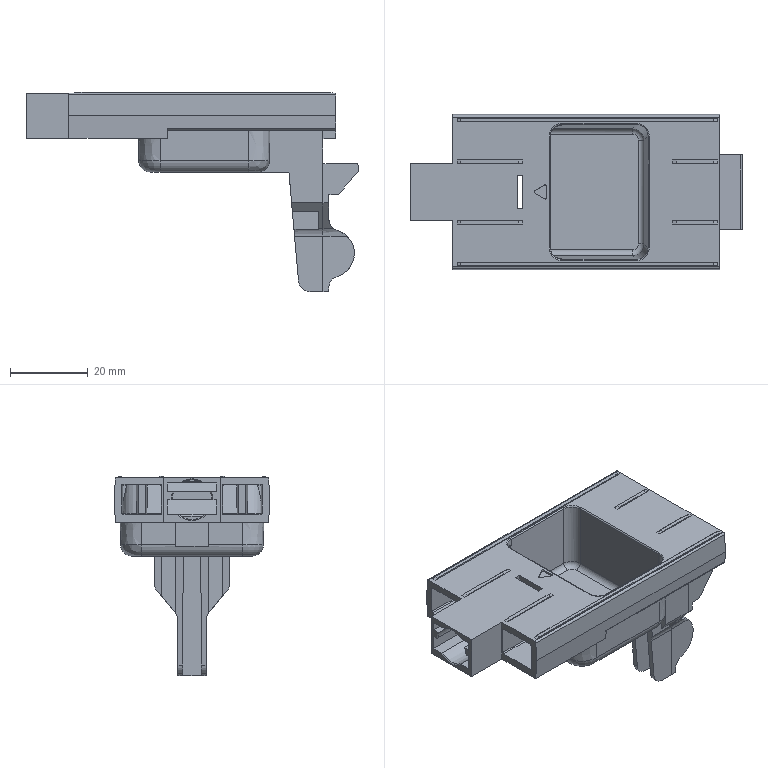Part | NX | features solid 2 | 1 solid | 269 faces | box 85.3 x 39.9 x 51.213 mm | volume 21117 mm3 | plane 188 | cylinder 53 | spline 15 | cone 10 | torus 3 | commonest cylinder face diameters 0.6 x17 6 x15 1 x6 3 x5 10.2 x4 6.016 x2